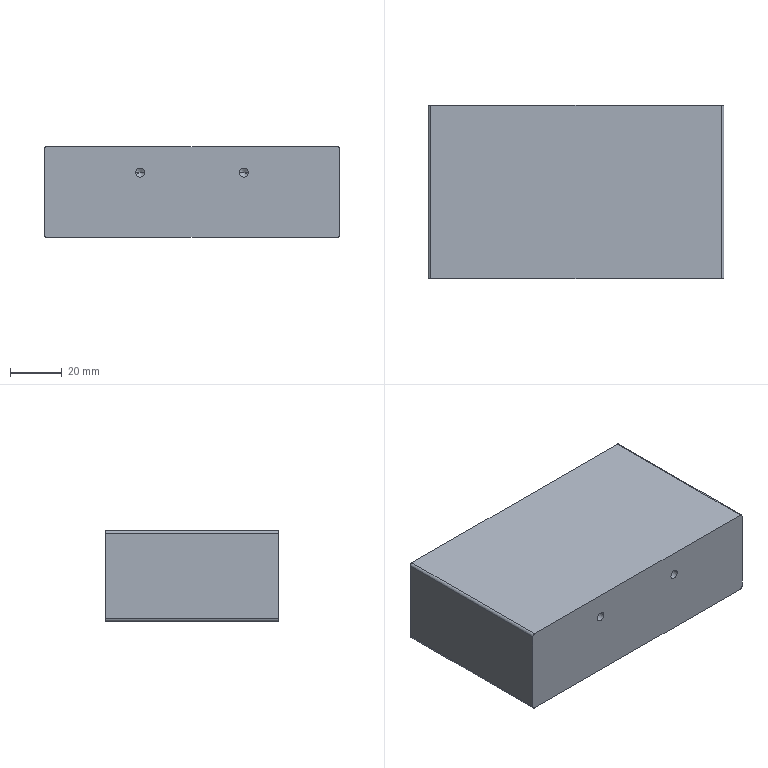NC program | NX | posted with a generic post | part box 114 x 67 x 35 mm
Whole program:
N10 G17 G21 G94 G90
(DRILLING_COPY_COPY , TOOL : D4A45)
N12 T02 M6
N14 G54
N16 G17 G0 G90 X17.5 Y-7.5 B0. C0. S5000 M3
N18 G43 Z30. H2
N20 G94 G81 G98 Z-1. F250. R3.
N22 X52.5
N24 X-52.5
N26 X-17.5
N28 G80
N30 G0 X-17.5 Y-7.5 Z30.
N32 M5
(DRILLING_COPY_COPY_COPY_COPY_COPY_COPY_COPY , TOOL : 3.5ZT)
N34 T15 M6
N36 G54
N38 G17 G0 G90 X52.5 Y-7.5 B0. C0. S1910 M3
N40 G43 Z30. H15
N42 G94 G83 G98 Z-11.552 F180. Q2. R3.
N44 X17.5
N46 X-17.5
N48 X-52.5
N50 G80
N52 G0 X-52.5 Y-7.5 Z30.
N54 M5
N56 M2